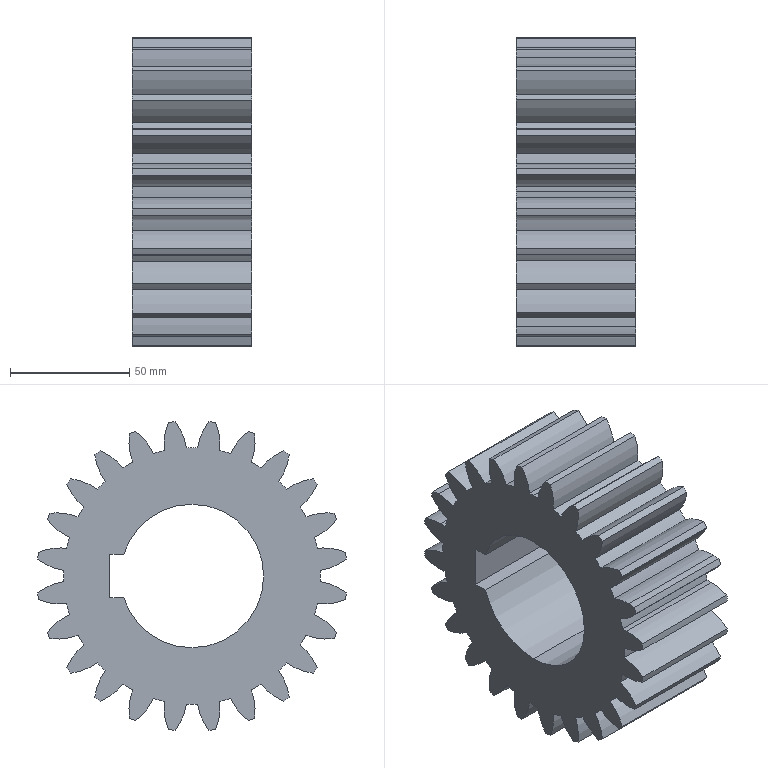Part | SolidWorks | features Boss 3, Cut 3, CirPattern 2, Fillet 2, Revolution 1 | 1 solid | 109 faces | box 50 x 129.229 x 129.229 mm | volume 404166 mm3 | cylinder 104 | plane 5 | commonest cylinder face diameters 48 x52 107.498 x25 130 x24 60 x3